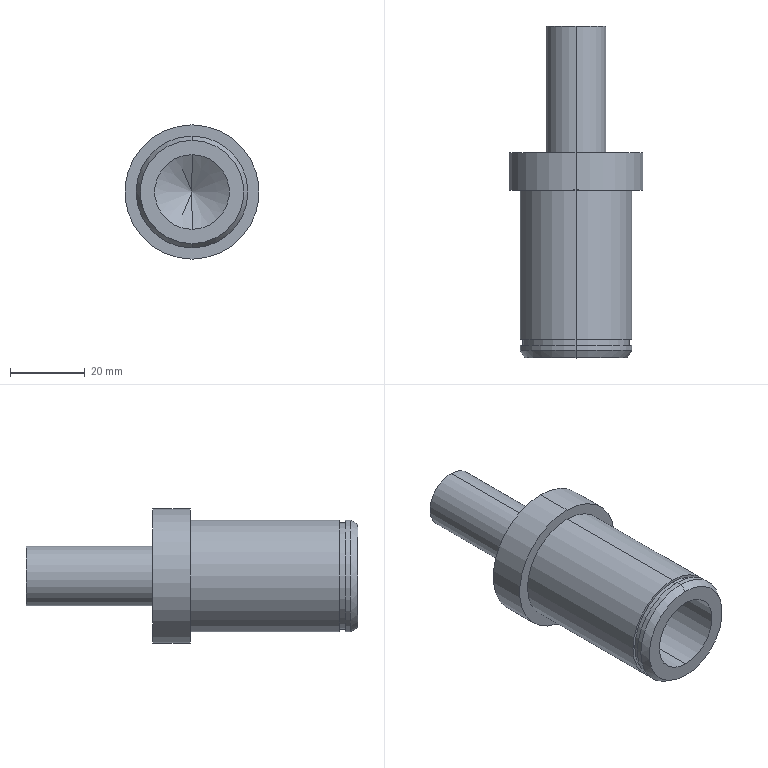Part | STEP file | 0229_221_Pin | 1 solid | 22 faces | box 36 x 89 x 36 mm | volume 38557 mm3 | cylinder 12 | plane 6 | cone 4 | commonest cylinder face diameters 30 x4 16 x2 20 x2 28.6 x2 36 x2
STEP:
#1=CARTESIAN_POINT('',(0.,0.,0.));
#2=DIRECTION('',(0.,0.,1.));
#3=DIRECTION('',(1.,0.,0.));
#4=AXIS2_PLACEMENT_3D('',#1,#2,#3);
#5=CARTESIAN_POINT('',(0.,-55.,-13.845));
#6=VERTEX_POINT('',#5);
#7=CARTESIAN_POINT('',(0.,-55.,13.845));
#8=VERTEX_POINT('',#7);
#9=CARTESIAN_POINT('',(0.,-55.,0.));
#10=DIRECTION('',(0.,-1.,0.));
#11=DIRECTION('',(0.,0.,1.));
#12=AXIS2_PLACEMENT_3D('',#9,#10,#11);
#13=CIRCLE('',#12,13.845);
#14=CARTESIAN_POINT('',(0.,-55.,0.));
#15=DIRECTION('',(0.,1.,0.));
#16=DIRECTION('',(0.,0.,1.));
#17=AXIS2_PLACEMENT_3D('',#14,#15,#16);
#18=CONICAL_SURFACE('',#17,13.845,0.5236);
#19=CARTESIAN_POINT('',(6.283,0.));
#20=DIRECTION('',(-1.,0.));
#21=VECTOR('',#20,1.);
#22=LINE('',#19,#21);
#23=(GEOMETRIC_REPRESENTATION_CONTEXT(2)PARAMETRIC_REPRESENTATION_CONTEXT()REPRESENTATION_CONTEXT('',''));
#24=DEFINITIONAL_REPRESENTATION('',(#22),#23);
#25=PCURVE('',#18,#24);
#26=CARTESIAN_POINT('',(-15.,-55.,0.));
#27=DIRECTION('',(0.,1.,0.));
#28=DIRECTION('',(0.,0.,1.));
#29=AXIS2_PLACEMENT_3D('',#26,#27,#28);
#30=PLANE('',#29);
#31=CARTESIAN_POINT('',(13.845,15.));
#32=CARTESIAN_POINT('',(13.845,-8.981));
#33=CARTESIAN_POINT('',(-6.923,3.01));
#34=CARTESIAN_POINT('',(-27.691,15.));
#35=CARTESIAN_POINT('',(-6.923,26.99));
#36=CARTESIAN_POINT('',(13.845,38.981));
#37=CARTESIAN_POINT('',(13.845,15.));
#38=(BOUNDED_CURVE()B_SPLINE_CURVE(2,(#31,#32,#33,#34,#35,#36,#37),.UNSPECIFIED.,.T.,.F.)B_SPLINE_CURVE_WITH_KNOTS((1,2,2,2,2,1),(-2.094,0.,2.094,4.189,6.283,8.378),.UNSPECIFIED.)CURVE()GEOMETRIC_REPRESENTATION_ITEM()RATIONAL_B_SPLINE_CURVE((1.,0.5,1.,0.5,1.,0.5,1.))REPRESENTATION_ITEM(''));
#39=(GEOMETRIC_REPRESENTATION_CONTEXT(2)PARAMETRIC_REPRESENTATION_CONTEXT()REPRESENTATION_CONTEXT('',''));
#40=DEFINITIONAL_REPRESENTATION('',(#38),#39);
#41=PCURVE('',#30,#40);
#42=SURFACE_CURVE('',#13,(#25,#41),.PCURVE_S1.);
#43=EDGE_CURVE('',#6,#8,#42,.T.);
#44=ORIENTED_EDGE('',*,*,#43,.F.);
#45=CARTESIAN_POINT('',(0.,-53.,-15.));
#46=VERTEX_POINT('',#45);
#47=CARTESIAN_POINT('',(0.,-55.,-13.845));
#48=DIRECTION('',(0.,0.866,-0.5));
#49=VECTOR('',#48,1.);
#50=LINE('',#47,#49);
#51=CARTESIAN_POINT('',(3.142,0.));
#52=DIRECTION('',(0.,1.));
#53=VECTOR('',#52,1.);
#54=LINE('',#51,#53);
#55=(GEOMETRIC_REPRESENTATION_CONTEXT(2)PARAMETRIC_REPRESENTATION_CONTEXT()REPRESENTATION_CONTEXT('',''));
#56=DEFINITIONAL_REPRESENTATION('',(#54),#55);
#57=PCURVE('',#18,#56);
#58=CARTESIAN_POINT('',(0.,-55.,0.));
#59=DIRECTION('',(0.,1.,0.));
#60=DIRECTION('',(0.,0.,1.));
#61=AXIS2_PLACEMENT_3D('',#58,#59,#60);
#62=CONICAL_SURFACE('',#61,13.845,0.5236);
#63=CARTESIAN_POINT('',(3.142,0.));
#64=DIRECTION('',(0.,1.));
#65=VECTOR('',#64,1.);
#66=LINE('',#63,#65);
#67=(GEOMETRIC_REPRESENTATION_CONTEXT(2)PARAMETRIC_REPRESENTATION_CONTEXT()REPRESENTATION_CONTEXT('',''));
#68=DEFINITIONAL_REPRESENTATION('',(#66),#67);
#69=PCURVE('',#62,#68);
#70=SURFACE_CURVE('',#50,(#57,#69),.PCURVE_S1.);
#71=EDGE_CURVE('',#6,#46,#70,.T.);
#72=ORIENTED_EDGE('',*,*,#71,.T.);
#73=CARTESIAN_POINT('',(0.,-53.,15.));
#74=VERTEX_POINT('',#73);
#75=CARTESIAN_POINT('',(0.,-53.,0.));
#76=DIRECTION('',(0.,1.,0.));
#77=DIRECTION('',(0.,0.,1.));
#78=AXIS2_PLACEMENT_3D('',#75,#76,#77);
#79=CIRCLE('',#78,15.);
#80=CARTESIAN_POINT('',(0.,2.));
#81=DIRECTION('',(1.,0.));
#82=VECTOR('',#81,1.);
#83=LINE('',#80,#82);
#84=(GEOMETRIC_REPRESENTATION_CONTEXT(2)PARAMETRIC_REPRESENTATION_CONTEXT()REPRESENTATION_CONTEXT('',''));
#85=DEFINITIONAL_REPRESENTATION('',(#83),#84);
#86=PCURVE('',#18,#85);
#87=CARTESIAN_POINT('',(0.,-62.558,0.));
#88=DIRECTION('',(0.,-1.,0.));
#89=DIRECTION('',(0.,0.,-1.));
#90=AXIS2_PLACEMENT_3D('',#87,#88,#89);
#91=CYLINDRICAL_SURFACE('',#90,15.);
#92=CARTESIAN_POINT('',(3.142,-9.558));
#93=DIRECTION('',(-1.,0.));
#94=VECTOR('',#93,1.);
#95=LINE('',#92,#94);
#96=(GEOMETRIC_REPRESENTATION_CONTEXT(2)PARAMETRIC_REPRESENTATION_CONTEXT()REPRESENTATION_CONTEXT('',''));
#97=DEFINITIONAL_REPRESENTATION('',(#95),#96);
#98=PCURVE('',#91,#97);
#99=SURFACE_CURVE('',#79,(#86,#98),.PCURVE_S1.);
#100=EDGE_CURVE('',#74,#46,#99,.T.);
#101=ORIENTED_EDGE('',*,*,#100,.F.);
#102=CARTESIAN_POINT('',(0.,-55.,13.845));
#103=DIRECTION('',(0.,0.866,0.5));
#104=VECTOR('',#103,1.);
#105=LINE('',#102,#104);
#106=CARTESIAN_POINT('',(0.,0.));
#107=DIRECTION('',(0.,1.));
#108=VECTOR('',#107,1.);
#109=LINE('',#106,#108);
#110=(GEOMETRIC_REPRESENTATION_CONTEXT(2)PARAMETRIC_REPRESENTATION_CONTEXT()REPRESENTATION_CONTEXT('',''));
#111=DEFINITIONAL_REPRESENTATION('',(#109),#110);
#112=PCURVE('',#18,#111);
#113=CARTESIAN_POINT('',(6.283,0.));
#114=DIRECTION('',(0.,1.));
#115=VECTOR('',#114,1.);
#116=LINE('',#113,#115);
#117=(GEOMETRIC_REPRESENTATION_CONTEXT(2)PARAMETRIC_REPRESENTATION_CONTEXT()REPRESENTATION_CONTEXT('',''));
#118=DEFINITIONAL_REPRESENTATION('',(#116),#117);
#119=PCURVE('',#62,#118);
#120=SURFACE_CURVE('',#105,(#112,#119),.PCURVE_S1.);
#121=EDGE_CURVE('',#8,#74,#120,.T.);
#122=ORIENTED_EDGE('',*,*,#121,.F.);
#123=EDGE_LOOP('',(#44,#72,#101,#122));
#124=FACE_BOUND('',#123,.T.);
#125=ADVANCED_FACE('',(#124),#18,.T.);
#126=CARTESIAN_POINT('',(0.,-25.,-10.));
#127=VERTEX_POINT('',#126);
#128=CARTESIAN_POINT('',(0.,-55.,-10.));
#129=VERTEX_POINT('',#128);
#130=CARTESIAN_POINT('',(0.,-55.,-10.));
#131=DIRECTION('',(0.,-1.,0.));
#132=VECTOR('',#131,1.);
#133=LINE('',#130,#132);
#134=CARTESIAN_POINT('',(0.,-55.,0.));
#135=DIRECTION('',(0.,-1.,0.));
#136=DIRECTION('',(0.,0.,-1.));
#137=AXIS2_PLACEMENT_3D('',#134,#135,#136);
#138=CYLINDRICAL_SURFACE('',#137,10.);
#139=CARTESIAN_POINT('',(6.283,0.));
#140=DIRECTION('',(0.,1.));
#141=VECTOR('',#140,1.);
#142=LINE('',#139,#141);
#143=(GEOMETRIC_REPRESENTATION_CONTEXT(2)PARAMETRIC_REPRESENTATION_CONTEXT()REPRESENTATION_CONTEXT('',''));
#144=DEFINITIONAL_REPRESENTATION('',(#142),#143);
#145=PCURVE('',#138,#144);
#146=CARTESIAN_POINT('',(0.,-55.,0.));
#147=DIRECTION('',(0.,-1.,0.));
#148=DIRECTION('',(0.,0.,-1.));
#149=AXIS2_PLACEMENT_3D('',#146,#147,#148);
#150=CYLINDRICAL_SURFACE('',#149,10.);
#151=CARTESIAN_POINT('',(0.,0.));
#152=DIRECTION('',(0.,1.));
#153=VECTOR('',#152,1.);
#154=LINE('',#151,#153);
#155=(GEOMETRIC_REPRESENTATION_CONTEXT(2)PARAMETRIC_REPRESENTATION_CONTEXT()REPRESENTATION_CONTEXT('',''));
#156=DEFINITIONAL_REPRESENTATION('',(#154),#155);
#157=PCURVE('',#150,#156);
#158=SURFACE_CURVE('',#133,(#145,#157),.PCURVE_S1.);
#159=EDGE_CURVE('',#127,#129,#158,.T.);
#160=ORIENTED_EDGE('',*,*,#159,.T.);
#161=CARTESIAN_POINT('',(0.,-55.,10.));
#162=VERTEX_POINT('',#161);
#163=CARTESIAN_POINT('',(0.,-55.,0.));
#164=DIRECTION('',(0.,-1.,0.));
#165=DIRECTION('',(0.,0.,-1.));
#166=AXIS2_PLACEMENT_3D('',#163,#164,#165);
#167=CIRCLE('',#166,10.);
#168=CARTESIAN_POINT('',(0.,0.));
#169=DIRECTION('',(1.,0.));
#170=VECTOR('',#169,1.);
#171=LINE('',#168,#170);
#172=(GEOMETRIC_REPRESENTATION_CONTEXT(2)PARAMETRIC_REPRESENTATION_CONTEXT()REPRESENTATION_CONTEXT('',''));
#173=DEFINITIONAL_REPRESENTATION('',(#171),#172);
#174=PCURVE('',#138,#173);
#175=CARTESIAN_POINT('',(-10.,15.));
#176=CARTESIAN_POINT('',(-10.,32.321));
#177=CARTESIAN_POINT('',(5.,23.66));
#178=CARTESIAN_POINT('',(20.,15.));
#179=CARTESIAN_POINT('',(5.,6.34));
#180=CARTESIAN_POINT('',(-10.,-2.321));
#181=CARTESIAN_POINT('',(-10.,15.));
#182=(BOUNDED_CURVE()B_SPLINE_CURVE(2,(#175,#176,#177,#178,#179,#180,#181),.UNSPECIFIED.,.T.,.F.)B_SPLINE_CURVE_WITH_KNOTS((1,2,2,2,2,1),(-2.094,0.,2.094,4.189,6.283,8.378),.UNSPECIFIED.)CURVE()GEOMETRIC_REPRESENTATION_ITEM()RATIONAL_B_SPLINE_CURVE((1.,0.5,1.,0.5,1.,0.5,1.))REPRESENTATION_ITEM(''));
#183=(GEOMETRIC_REPRESENTATION_CONTEXT(2)PARAMETRIC_REPRESENTATION_CONTEXT()REPRESENTATION_CONTEXT('',''));
#184=DEFINITIONAL_REPRESENTATION('',(#182),#183);
#185=PCURVE('',#30,#184);
#186=SURFACE_CURVE('',#167,(#174,#185),.PCURVE_S1.);
#187=EDGE_CURVE('',#162,#129,#186,.T.);
#188=ORIENTED_EDGE('',*,*,#187,.F.);
#189=CARTESIAN_POINT('',(0.,-25.,10.));
#190=VERTEX_POINT('',#189);
#191=CARTESIAN_POINT('',(0.,-55.,10.));
#192=DIRECTION('',(0.,-1.,0.));
#193=VECTOR('',#192,1.);
#194=LINE('',#191,#193);
#195=CARTESIAN_POINT('',(3.142,0.));
#196=DIRECTION('',(0.,1.));
#197=VECTOR('',#196,1.);
#198=LINE('',#195,#197);
#199=(GEOMETRIC_REPRESENTATION_CONTEXT(2)PARAMETRIC_REPRESENTATION_CONTEXT()REPRESENTATION_CONTEXT('',''));
#200=DEFINITIONAL_REPRESENTATION('',(#198),#199);
#201=PCURVE('',#138,#200);
#202=CARTESIAN_POINT('',(3.142,0.));
#203=DIRECTION('',(0.,1.));
#204=VECTOR('',#203,1.);
#205=LINE('',#202,#204);
#206=(GEOMETRIC_REPRESENTATION_CONTEXT(2)PARAMETRIC_REPRESENTATION_CONTEXT()REPRESENTATION_CONTEXT('',''));
#207=DEFINITIONAL_REPRESENTATION('',(#205),#206);
#208=PCURVE('',#150,#207);
#209=SURFACE_CURVE('',#194,(#201,#208),.PCURVE_S1.);
#210=EDGE_CURVE('',#190,#162,#209,.T.);
#211=ORIENTED_EDGE('',*,*,#210,.F.);
#212=CARTESIAN_POINT('',(0.,-25.,0.));
#213=DIRECTION('',(0.,-1.,0.));
#214=DIRECTION('',(0.,0.,-1.));
#215=AXIS2_PLACEMENT_3D('',#212,#213,#214);
#216=CIRCLE('',#215,10.);
#217=CARTESIAN_POINT('',(0.,-30.));
#218=DIRECTION('',(1.,0.));
#219=VECTOR('',#218,1.);
#220=LINE('',#217,#219);
#221=(GEOMETRIC_REPRESENTATION_CONTEXT(2)PARAMETRIC_REPRESENTATION_CONTEXT()REPRESENTATION_CONTEXT('',''));
#222=DEFINITIONAL_REPRESENTATION('',(#220),#221);
#223=PCURVE('',#138,#222);
#224=CARTESIAN_POINT('',(0.,-25.,0.));
#225=DIRECTION('',(0.,-1.,0.));
#226=DIRECTION('',(0.,0.,-1.));
#227=AXIS2_PLACEMENT_3D('',#224,#225,#226);
#228=CONICAL_SURFACE('',#227,10.,1.03);
#229=CARTESIAN_POINT('',(0.,0.));
#230=DIRECTION('',(1.,0.));
#231=VECTOR('',#230,1.);
#232=LINE('',#229,#231);
#233=(GEOMETRIC_REPRESENTATION_CONTEXT(2)PARAMETRIC_REPRESENTATION_CONTEXT()REPRESENTATION_CONTEXT('',''));
#234=DEFINITIONAL_REPRESENTATION('',(#232),#233);
#235=PCURVE('',#228,#234);
#236=SURFACE_CURVE('',#216,(#223,#235),.PCURVE_S1.);
#237=EDGE_CURVE('',#190,#127,#236,.T.);
#238=ORIENTED_EDGE('',*,*,#237,.T.);
#239=EDGE_LOOP('',(#160,#188,#211,#238));
#240=FACE_BOUND('',#239,.F.);
#241=ADVANCED_FACE('',(#240),#138,.F.);
#242=ORIENTED_EDGE('',*,*,#237,.F.);
#243=CARTESIAN_POINT('',(0.,-18.991,0.));
#244=VERTEX_POINT('',#243);
#245=CARTESIAN_POINT('',(0.,-25.,10.));
#246=DIRECTION('',(0.,-0.515,0.8572));
#247=VECTOR('',#246,1.);
#248=LINE('',#245,#247);
#249=CARTESIAN_POINT('',(3.142,0.));
#250=DIRECTION('',(0.,1.));
#251=VECTOR('',#250,1.);
#252=LINE('',#249,#251);
#253=(GEOMETRIC_REPRESENTATION_CONTEXT(2)PARAMETRIC_REPRESENTATION_CONTEXT()REPRESENTATION_CONTEXT('',''));
#254=DEFINITIONAL_REPRESENTATION('',(#252),#253);
#255=PCURVE('',#228,#254);
#256=CARTESIAN_POINT('',(0.,-25.,0.));
#257=DIRECTION('',(0.,-1.,0.));
#258=DIRECTION('',(0.,0.,-1.));
#259=AXIS2_PLACEMENT_3D('',#256,#257,#258);
#260=CONICAL_SURFACE('',#259,10.,1.03);
#261=CARTESIAN_POINT('',(3.142,0.));
#262=DIRECTION('',(0.,1.));
#263=VECTOR('',#262,1.);
#264=LINE('',#261,#263);
#265=(GEOMETRIC_REPRESENTATION_CONTEXT(2)PARAMETRIC_REPRESENTATION_CONTEXT()REPRESENTATION_CONTEXT('',''));
#266=DEFINITIONAL_REPRESENTATION('',(#264),#265);
#267=PCURVE('',#260,#266);
#268=SURFACE_CURVE('',#248,(#255,#267),.PCURVE_S1.);
#269=EDGE_CURVE('',#244,#190,#268,.T.);
#270=ORIENTED_EDGE('',*,*,#269,.F.);
#271=CARTESIAN_POINT('',(0.,-25.,-10.));
#272=DIRECTION('',(0.,-0.515,-0.8572));
#273=VECTOR('',#272,1.);
#274=LINE('',#271,#273);
#275=CARTESIAN_POINT('',(6.283,0.));
#276=DIRECTION('',(0.,1.));
#277=VECTOR('',#276,1.);
#278=LINE('',#275,#277);
#279=(GEOMETRIC_REPRESENTATION_CONTEXT(2)PARAMETRIC_REPRESENTATION_CONTEXT()REPRESENTATION_CONTEXT('',''));
#280=DEFINITIONAL_REPRESENTATION('',(#278),#279);
#281=PCURVE('',#228,#280);
#282=CARTESIAN_POINT('',(0.,0.));
#283=DIRECTION('',(0.,1.));
#284=VECTOR('',#283,1.);
#285=LINE('',#282,#284);
#286=(GEOMETRIC_REPRESENTATION_CONTEXT(2)PARAMETRIC_REPRESENTATION_CONTEXT()REPRESENTATION_CONTEXT('',''));
#287=DEFINITIONAL_REPRESENTATION('',(#285),#286);
#288=PCURVE('',#260,#287);
#289=SURFACE_CURVE('',#274,(#281,#288),.PCURVE_S1.);
#290=EDGE_CURVE('',#244,#127,#289,.T.);
#291=ORIENTED_EDGE('',*,*,#290,.T.);
#292=EDGE_LOOP('',(#242,#270,#291));
#293=FACE_BOUND('',#292,.F.);
#294=ADVANCED_FACE('',(#293),#228,.F.);
#295=CARTESIAN_POINT('',(0.,-10.,-15.));
#296=VERTEX_POINT('',#295);
#297=CARTESIAN_POINT('',(0.,-10.,15.));
#298=VERTEX_POINT('',#297);
#299=CARTESIAN_POINT('',(0.,-10.,0.));
#300=DIRECTION('',(0.,-1.,0.));
#301=DIRECTION('',(0.,0.,-1.));
#302=AXIS2_PLACEMENT_3D('',#299,#300,#301);
#303=CIRCLE('',#302,15.);
#304=CARTESIAN_POINT('',(0.,-62.558,0.));
#305=DIRECTION('',(0.,-1.,0.));
#306=DIRECTION('',(0.,0.,-1.));
#307=AXIS2_PLACEMENT_3D('',#304,#305,#306);
#308=CYLINDRICAL_SURFACE('',#307,15.);
#309=CARTESIAN_POINT('',(0.,-52.558));
#310=DIRECTION('',(1.,0.));
#311=VECTOR('',#310,1.);
#312=LINE('',#309,#311);
#313=(GEOMETRIC_REPRESENTATION_CONTEXT(2)PARAMETRIC_REPRESENTATION_CONTEXT()REPRESENTATION_CONTEXT('',''));
#314=DEFINITIONAL_REPRESENTATION('',(#312),#313);
#315=PCURVE('',#308,#314);
#316=CARTESIAN_POINT('',(-15.,-10.,0.));
#317=DIRECTION('',(0.,1.,0.));
#318=DIRECTION('',(0.,0.,1.));
#319=AXIS2_PLACEMENT_3D('',#316,#317,#318);
#320=PLANE('',#319);
#321=CARTESIAN_POINT('',(-15.,15.));
#322=CARTESIAN_POINT('',(-15.,40.981));
#323=CARTESIAN_POINT('',(7.5,27.99));
#324=CARTESIAN_POINT('',(30.,15.));
#325=CARTESIAN_POINT('',(7.5,2.01));
#326=CARTESIAN_POINT('',(-15.,-10.981));
#327=CARTESIAN_POINT('',(-15.,15.));
#328=(BOUNDED_CURVE()B_SPLINE_CURVE(2,(#321,#322,#323,#324,#325,#326,#327),.UNSPECIFIED.,.T.,.F.)B_SPLINE_CURVE_WITH_KNOTS((1,2,2,2,2,1),(-2.094,0.,2.094,4.189,6.283,8.378),.UNSPECIFIED.)CURVE()GEOMETRIC_REPRESENTATION_ITEM()RATIONAL_B_SPLINE_CURVE((1.,0.5,1.,0.5,1.,0.5,1.))REPRESENTATION_ITEM(''));
#329=(GEOMETRIC_REPRESENTATION_CONTEXT(2)PARAMETRIC_REPRESENTATION_CONTEXT()REPRESENTATION_CONTEXT('',''));
#330=DEFINITIONAL_REPRESENTATION('',(#328),#329);
#331=PCURVE('',#320,#330);
#332=SURFACE_CURVE('',#303,(#315,#331),.PCURVE_S1.);
#333=EDGE_CURVE('',#296,#298,#332,.T.);
#334=ORIENTED_EDGE('',*,*,#333,.T.);
#335=CARTESIAN_POINT('',(0.,-50.,15.));
#336=VERTEX_POINT('',#335);
#337=CARTESIAN_POINT('',(0.,-62.558,15.));
#338=DIRECTION('',(0.,-1.,0.));
#339=VECTOR('',#338,1.);
#340=LINE('',#337,#339);
#341=CARTESIAN_POINT('',(3.142,0.));
#342=DIRECTION('',(0.,1.));
#343=VECTOR('',#342,1.);
#344=LINE('',#341,#343);
#345=(GEOMETRIC_REPRESENTATION_CONTEXT(2)PARAMETRIC_REPRESENTATION_CONTEXT()REPRESENTATION_CONTEXT('',''));
#346=DEFINITIONAL_REPRESENTATION('',(#344),#345);
#347=PCURVE('',#308,#346);
#348=CARTESIAN_POINT('',(0.,-62.558,0.));
#349=DIRECTION('',(0.,-1.,0.));
#350=DIRECTION('',(0.,0.,-1.));
#351=AXIS2_PLACEMENT_3D('',#348,#349,#350);
#352=CYLINDRICAL_SURFACE('',#351,15.);
#353=CARTESIAN_POINT('',(3.142,0.));
#354=DIRECTION('',(0.,1.));
#355=VECTOR('',#354,1.);
#356=LINE('',#353,#355);
#357=(GEOMETRIC_REPRESENTATION_CONTEXT(2)PARAMETRIC_REPRESENTATION_CONTEXT()REPRESENTATION_CONTEXT('',''));
#358=DEFINITIONAL_REPRESENTATION('',(#356),#357);
#359=PCURVE('',#352,#358);
#360=SURFACE_CURVE('',#340,(#347,#359),.PCURVE_S1.);
#361=EDGE_CURVE('',#298,#336,#360,.T.);
#362=ORIENTED_EDGE('',*,*,#361,.T.);
#363=CARTESIAN_POINT('',(0.,-50.,-15.));
#364=VERTEX_POINT('',#363);
#365=CARTESIAN_POINT('',(0.,-50.,0.));
#366=DIRECTION('',(0.,-1.,0.));
#367=DIRECTION('',(0.,0.,-1.));
#368=AXIS2_PLACEMENT_3D('',#365,#366,#367);
#369=CIRCLE('',#368,15.);
#370=CARTESIAN_POINT('',(0.,-12.558));
#371=DIRECTION('',(1.,0.));
#372=VECTOR('',#371,1.);
#373=LINE('',#370,#372);
#374=(GEOMETRIC_REPRESENTATION_CONTEXT(2)PARAMETRIC_REPRESENTATION_CONTEXT()REPRESENTATION_CONTEXT('',''));
#375=DEFINITIONAL_REPRESENTATION('',(#373),#374);
#376=PCURVE('',#308,#375);
#377=CARTESIAN_POINT('',(-15.,-50.,0.));
#378=DIRECTION('',(0.,1.,0.));
#379=DIRECTION('',(0.,0.,1.));
#380=AXIS2_PLACEMENT_3D('',#377,#378,#379);
#381=PLANE('',#380);
#382=CARTESIAN_POINT('',(-15.,15.));
#383=CARTESIAN_POINT('',(-15.,40.981));
#384=CARTESIAN_POINT('',(7.5,27.99));
#385=CARTESIAN_POINT('',(30.,15.));
#386=CARTESIAN_POINT('',(7.5,2.01));
#387=CARTESIAN_POINT('',(-15.,-10.981));
#388=CARTESIAN_POINT('',(-15.,15.));
#389=(BOUNDED_CURVE()B_SPLINE_CURVE(2,(#382,#383,#384,#385,#386,#387,#388),.UNSPECIFIED.,.T.,.F.)B_SPLINE_CURVE_WITH_KNOTS((1,2,2,2,2,1),(-2.094,0.,2.094,4.189,6.283,8.378),.UNSPECIFIED.)CURVE()GEOMETRIC_REPRESENTATION_ITEM()RATIONAL_B_SPLINE_CURVE((1.,0.5,1.,0.5,1.,0.5,1.))REPRESENTATION_ITEM(''));
#390=(GEOMETRIC_REPRESENTATION_CONTEXT(2)PARAMETRIC_REPRESENTATION_CONTEXT()REPRESENTATION_CONTEXT('',''));
#391=DEFINITIONAL_REPRESENTATION('',(#389),#390);
#392=PCURVE('',#381,#391);
#393=SURFACE_CURVE('',#369,(#376,#392),.PCURVE_S1.);
#394=EDGE_CURVE('',#364,#336,#393,.T.);
#395=ORIENTED_EDGE('',*,*,#394,.F.);
#396=CARTESIAN_POINT('',(0.,-62.558,-15.));
#397=DIRECTION('',(0.,-1.,0.));
#398=VECTOR('',#397,1.);
#399=LINE('',#396,#398);
#400=CARTESIAN_POINT('',(0.,0.));
#401=DIRECTION('',(0.,1.));
#402=VECTOR('',#401,1.);
#403=LINE('',#400,#402);
#404=(GEOMETRIC_REPRESENTATION_CONTEXT(2)PARAMETRIC_REPRESENTATION_CONTEXT()REPRESENTATION_CONTEXT('',''));
#405=DEFINITIONAL_REPRESENTATION('',(#403),#404);
#406=PCURVE('',#308,#405);
#407=CARTESIAN_POINT('',(6.283,0.));
#408=DIRECTION('',(0.,1.));
#409=VECTOR('',#408,1.);
#410=LINE('',#407,#409);
#411=(GEOMETRIC_REPRESENTATION_CONTEXT(2)PARAMETRIC_REPRESENTATION_CONTEXT()REPRESENTATION_CONTEXT('',''));
#412=DEFINITIONAL_REPRESENTATION('',(#410),#411);
#413=PCURVE('',#352,#412);
#414=SURFACE_CURVE('',#399,(#406,#413),.PCURVE_S1.);
#415=EDGE_CURVE('',#296,#364,#414,.T.);
#416=ORIENTED_EDGE('',*,*,#415,.F.);
#417=EDGE_LOOP('',(#334,#362,#395,#416));
#418=FACE_BOUND('',#417,.T.);
#419=ADVANCED_FACE('',(#418),#308,.T.);
#420=CARTESIAN_POINT('',(0.,-50.,-14.3));
#421=VERTEX_POINT('',#420);
#422=CARTESIAN_POINT('',(0.,-50.,14.3));
#423=VERTEX_POINT('',#422);
#424=CARTESIAN_POINT('',(0.,-50.,0.));
#425=DIRECTION('',(0.,-1.,0.));
#426=DIRECTION('',(0.,0.,-1.));
#427=AXIS2_PLACEMENT_3D('',#424,#425,#426);
#428=CIRCLE('',#427,14.3);
#429=CARTESIAN_POINT('',(0.,-62.558,0.));
#430=DIRECTION('',(0.,-1.,0.));
#431=DIRECTION('',(0.,0.,-1.));
#432=AXIS2_PLACEMENT_3D('',#429,#430,#431);
#433=CYLINDRICAL_SURFACE('',#432,14.3);
#434=CARTESIAN_POINT('',(0.,-12.558));
#435=DIRECTION('',(1.,0.));
#436=VECTOR('',#435,1.);
#437=LINE('',#434,#436);
#438=(GEOMETRIC_REPRESENTATION_CONTEXT(2)PARAMETRIC_REPRESENTATION_CONTEXT()REPRESENTATION_CONTEXT('',''));
#439=DEFINITIONAL_REPRESENTATION('',(#437),#438);
#440=PCURVE('',#433,#439);
#441=CARTESIAN_POINT('',(-14.3,15.));
#442=CARTESIAN_POINT('',(-14.3,39.768));
#443=CARTESIAN_POINT('',(7.15,27.384));
#444=CARTESIAN_POINT('',(28.6,15.));
#445=CARTESIAN_POINT('',(7.15,2.616));
#446=CARTESIAN_POINT('',(-14.3,-9.768));
#447=CARTESIAN_POINT('',(-14.3,15.));
#448=(BOUNDED_CURVE()B_SPLINE_CURVE(2,(#441,#442,#443,#444,#445,#446,#447),.UNSPECIFIED.,.T.,.F.)B_SPLINE_CURVE_WITH_KNOTS((1,2,2,2,2,1),(-2.094,0.,2.094,4.189,6.283,8.378),.UNSPECIFIED.)CURVE()GEOMETRIC_REPRESENTATION_ITEM()RATIONAL_B_SPLINE_CURVE((1.,0.5,1.,0.5,1.,0.5,1.))REPRESENTATION_ITEM(''));
#449=(GEOMETRIC_REPRESENTATION_CONTEXT(2)PARAMETRIC_REPRESENTATION_CONTEXT()REPRESENTATION_CONTEXT('',''));
#450=DEFINITIONAL_REPRESENTATION('',(#448),#449);
#451=PCURVE('',#381,#450);
#452=SURFACE_CURVE('',#428,(#440,#451),.PCURVE_S1.);
#453=EDGE_CURVE('',#421,#423,#452,.T.);
#454=ORIENTED_EDGE('',*,*,#453,.T.);
#455=CARTESIAN_POINT('',(0.,-51.65,14.3));
#456=VERTEX_POINT('',#455);
#457=CARTESIAN_POINT('',(0.,-62.558,14.3));
#458=DIRECTION('',(0.,-1.,0.));
#459=VECTOR('',#458,1.);
#460=LINE('',#457,#459);
#461=CARTESIAN_POINT('',(3.142,0.));
#462=DIRECTION('',(0.,1.));
#463=VECTOR('',#462,1.);
#464=LINE('',#461,#463);
#465=(GEOMETRIC_REPRESENTATION_CONTEXT(2)PARAMETRIC_REPRESENTATION_CONTEXT()REPRESENTATION_CONTEXT('',''));
#466=DEFINITIONAL_REPRESENTATION('',(#464),#465);
#467=PCURVE('',#433,#466);
#468=CARTESIAN_POINT('',(0.,-62.558,0.));
#469=DIRECTION('',(0.,-1.,0.));
#470=DIRECTION('',(0.,0.,-1.));
#471=AXIS2_PLACEMENT_3D('',#468,#469,#470);
#472=CYLINDRICAL_SURFACE('',#471,14.3);
#473=CARTESIAN_POINT('',(3.142,0.));
#474=DIRECTION('',(0.,1.));
#475=VECTOR('',#474,1.);
#476=LINE('',#473,#475);
#477=(GEOMETRIC_REPRESENTATION_CONTEXT(2)PARAMETRIC_REPRESENTATION_CONTEXT()REPRESENTATION_CONTEXT('',''));
#478=DEFINITIONAL_REPRESENTATION('',(#476),#477);
#479=PCURVE('',#472,#478);
#480=SURFACE_CURVE('',#460,(#467,#479),.PCURVE_S1.);
#481=EDGE_CURVE('',#423,#456,#480,.T.);
#482=ORIENTED_EDGE('',*,*,#481,.T.);
#483=CARTESIAN_POINT('',(0.,-51.65,-14.3));
#484=VERTEX_POINT('',#483);
#485=CARTESIAN_POINT('',(0.,-51.65,0.));
#486=DIRECTION('',(0.,-1.,0.));
#487=DIRECTION('',(0.,0.,-1.));
#488=AXIS2_PLACEMENT_3D('',#485,#486,#487);
#489=CIRCLE('',#488,14.3);
#490=CARTESIAN_POINT('',(0.,-10.908));
#491=DIRECTION('',(1.,0.));
#492=VECTOR('',#491,1.);
#493=LINE('',#490,#492);
#494=(GEOMETRIC_REPRESENTATION_CONTEXT(2)PARAMETRIC_REPRESENTATION_CONTEXT()REPRESENTATION_CONTEXT('',''));
#495=DEFINITIONAL_REPRESENTATION('',(#493),#494);
#496=PCURVE('',#433,#495);
#497=CARTESIAN_POINT('',(-15.,-51.65,0.));
#498=DIRECTION('',(0.,-1.,0.));
#499=DIRECTION('',(0.,0.,-1.));
#500=AXIS2_PLACEMENT_3D('',#497,#498,#499);
#501=PLANE('',#500);
#502=CARTESIAN_POINT('',(0.,15.));
#503=DIRECTION('',(1.,0.));
#504=AXIS2_PLACEMENT_2D('',#502,#503);
#505=CIRCLE('',#504,14.3);
#506=(GEOMETRIC_REPRESENTATION_CONTEXT(2)PARAMETRIC_REPRESENTATION_CONTEXT()REPRESENTATION_CONTEXT('',''));
#507=DEFINITIONAL_REPRESENTATION('',(#505),#506);
#508=PCURVE('',#501,#507);
#509=SURFACE_CURVE('',#489,(#496,#508),.PCURVE_S1.);
#510=EDGE_CURVE('',#484,#456,#509,.T.);
#511=ORIENTED_EDGE('',*,*,#510,.F.);
#512=CARTESIAN_POINT('',(0.,-62.558,-14.3));
#513=DIRECTION('',(0.,-1.,0.));
#514=VECTOR('',#513,1.);
#515=LINE('',#512,#514);
#516=CARTESIAN_POINT('',(0.,0.));
#517=DIRECTION('',(0.,1.));
#518=VECTOR('',#517,1.);
#519=LINE('',#516,#518);
#520=(GEOMETRIC_REPRESENTATION_CONTEXT(2)PARAMETRIC_REPRESENTATION_CONTEXT()REPRESENTATION_CONTEXT('',''));
#521=DEFINITIONAL_REPRESENTATION('',(#519),#520);
#522=PCURVE('',#433,#521);
#523=CARTESIAN_POINT('',(6.283,0.));
#524=DIRECTION('',(0.,1.));
#525=VECTOR('',#524,1.);
#526=LINE('',#523,#525);
#527=(GEOMETRIC_REPRESENTATION_CONTEXT(2)PARAMETRIC_REPRESENTATION_CONTEXT()REPRESENTATION_CONTEXT('',''));
#528=DEFINITIONAL_REPRESENTATION('',(#526),#527);
#529=PCURVE('',#472,#528);
#530=SURFACE_CURVE('',#515,(#522,#529),.PCURVE_S1.);
#531=EDGE_CURVE('',#421,#484,#530,.T.);
#532=ORIENTED_EDGE('',*,*,#531,.F.);
#533=EDGE_LOOP('',(#454,#482,#511,#532));
#534=FACE_BOUND('',#533,.T.);
#535=ADVANCED_FACE('',(#534),#433,.T.);
#536=CARTESIAN_POINT('',(0.,-51.65,-15.));
#537=VERTEX_POINT('',#536);
#538=CARTESIAN_POINT('',(0.,-51.65,15.));
#539=VERTEX_POINT('',#538);
#540=CARTESIAN_POINT('',(0.,-51.65,0.));
#541=DIRECTION('',(0.,-1.,0.));
#542=DIRECTION('',(0.,0.,-1.));
#543=AXIS2_PLACEMENT_3D('',#540,#541,#542);
#544=CIRCLE('',#543,15.);
#545=CARTESIAN_POINT('',(0.,-10.908));
#546=DIRECTION('',(1.,0.));
#547=VECTOR('',#546,1.);
#548=LINE('',#545,#547);
#549=(GEOMETRIC_REPRESENTATION_CONTEXT(2)PARAMETRIC_REPRESENTATION_CONTEXT()REPRESENTATION_CONTEXT('',''));
#550=DEFINITIONAL_REPRESENTATION('',(#548),#549);
#551=PCURVE('',#91,#550);
#552=CARTESIAN_POINT('',(0.,15.));
#553=DIRECTION('',(1.,0.));
#554=AXIS2_PLACEMENT_2D('',#552,#553);
#555=CIRCLE('',#554,15.);
#556=(GEOMETRIC_REPRESENTATION_CONTEXT(2)PARAMETRIC_REPRESENTATION_CONTEXT()REPRESENTATION_CONTEXT('',''));
#557=DEFINITIONAL_REPRESENTATION('',(#555),#556);
#558=PCURVE('',#501,#557);
#559=SURFACE_CURVE('',#544,(#551,#558),.PCURVE_S1.);
#560=EDGE_CURVE('',#537,#539,#559,.T.);
#561=ORIENTED_EDGE('',*,*,#560,.T.);
#562=CARTESIAN_POINT('',(0.,-62.558,15.));
#563=DIRECTION('',(0.,-1.,0.));
#564=VECTOR('',#563,1.);
#565=LINE('',#562,#564);
#566=CARTESIAN_POINT('',(3.142,0.));
#567=DIRECTION('',(0.,1.));
#568=VECTOR('',#567,1.);
#569=LINE('',#566,#568);
#570=(GEOMETRIC_REPRESENTATION_CONTEXT(2)PARAMETRIC_REPRESENTATION_CONTEXT()REPRESENTATION_CONTEXT('',''));
#571=DEFINITIONAL_REPRESENTATION('',(#569),#570);
#572=PCURVE('',#91,#571);
#573=CARTESIAN_POINT('',(0.,-62.558,0.));
#574=DIRECTION('',(0.,-1.,0.));
#575=DIRECTION('',(0.,0.,-1.));
#576=AXIS2_PLACEMENT_3D('',#573,#574,#575);
#577=CYLINDRICAL_SURFACE('',#576,15.);
#578=CARTESIAN_POINT('',(3.142,0.));
#579=DIRECTION('',(0.,1.));
#580=VECTOR('',#579,1.);
#581=LINE('',#578,#580);
#582=(GEOMETRIC_REPRESENTATION_CONTEXT(2)PARAMETRIC_REPRESENTATION_CONTEXT()REPRESENTATION_CONTEXT('',''));
#583=DEFINITIONAL_REPRESENTATION('',(#581),#582);
#584=PCURVE('',#577,#583);
#585=SURFACE_CURVE('',#565,(#572,#584),.PCURVE_S1.);
#586=EDGE_CURVE('',#539,#74,#585,.T.);
#587=ORIENTED_EDGE('',*,*,#586,.T.);
#588=ORIENTED_EDGE('',*,*,#100,.T.);
#589=CARTESIAN_POINT('',(0.,-62.558,-15.));
#590=DIRECTION('',(0.,-1.,0.));
#591=VECTOR('',#590,1.);
#592=LINE('',#589,#591);
#593=CARTESIAN_POINT('',(0.,0.));
#594=DIRECTION('',(0.,1.));
#595=VECTOR('',#594,1.);
#596=LINE('',#593,#595);
#597=(GEOMETRIC_REPRESENTATION_CONTEXT(2)PARAMETRIC_REPRESENTATION_CONTEXT()REPRESENTATION_CONTEXT('',''));
#598=DEFINITIONAL_REPRESENTATION('',(#596),#597);
#599=PCURVE('',#91,#598);
#600=CARTESIAN_POINT('',(6.283,0.));
#601=DIRECTION('',(0.,1.));
#602=VECTOR('',#601,1.);
#603=LINE('',#600,#602);
#604=(GEOMETRIC_REPRESENTATION_CONTEXT(2)PARAMETRIC_REPRESENTATION_CONTEXT()REPRESENTATION_CONTEXT('',''));
#605=DEFINITIONAL_REPRESENTATION('',(#603),#604);
#606=PCURVE('',#577,#605);
#607=SURFACE_CURVE('',#592,(#599,#606),.PCURVE_S1.);
#608=EDGE_CURVE('',#537,#46,#607,.T.);
#609=ORIENTED_EDGE('',*,*,#608,.F.);
#610=EDGE_LOOP('',(#561,#587,#588,#609));
#611=FACE_BOUND('',#610,.T.);
#612=ADVANCED_FACE('',(#611),#91,.T.);
#613=CARTESIAN_POINT('',(0.,34.,-8.));
#614=VERTEX_POINT('',#613);
#615=CARTESIAN_POINT('',(0.,34.,8.));
#616=VERTEX_POINT('',#615);
#617=CARTESIAN_POINT('',(0.,34.,0.));
#618=DIRECTION('',(0.,-1.,0.));
#619=DIRECTION('',(0.,0.,-1.));
#620=AXIS2_PLACEMENT_3D('',#617,#618,#619);
#621=CIRCLE('',#620,8.);
#622=CARTESIAN_POINT('',(0.,-62.558,0.));
#623=DIRECTION('',(0.,-1.,0.));
#624=DIRECTION('',(0.,0.,-1.));
#625=AXIS2_PLACEMENT_3D('',#622,#623,#624);
#626=CYLINDRICAL_SURFACE('',#625,8.);
#627=CARTESIAN_POINT('',(0.,-96.558));
#628=DIRECTION('',(1.,0.));
#629=VECTOR('',#628,1.);
#630=LINE('',#627,#629);
#631=(GEOMETRIC_REPRESENTATION_CONTEXT(2)PARAMETRIC_REPRESENTATION_CONTEXT()REPRESENTATION_CONTEXT('',''));
#632=DEFINITIONAL_REPRESENTATION('',(#630),#631);
#633=PCURVE('',#626,#632);
#634=CARTESIAN_POINT('',(0.,34.,0.));
#635=DIRECTION('',(0.,-1.,0.));
#636=DIRECTION('',(0.,0.,-1.));
#637=AXIS2_PLACEMENT_3D('',#634,#635,#636);
#638=PLANE('',#637);
#639=CARTESIAN_POINT('',(0.,0.));
#640=DIRECTION('',(1.,0.));
#641=AXIS2_PLACEMENT_2D('',#639,#640);
#642=CIRCLE('',#641,8.);
#643=(GEOMETRIC_REPRESENTATION_CONTEXT(2)PARAMETRIC_REPRESENTATION_CONTEXT()REPRESENTATION_CONTEXT('',''));
#644=DEFINITIONAL_REPRESENTATION('',(#642),#643);
#645=PCURVE('',#638,#644);
#646=SURFACE_CURVE('',#621,(#633,#645),.PCURVE_S1.);
#647=EDGE_CURVE('',#614,#616,#646,.T.);
#648=ORIENTED_EDGE('',*,*,#647,.T.);
#649=CARTESIAN_POINT('',(0.,0.,8.));
#650=VERTEX_POINT('',#649);
#651=CARTESIAN_POINT('',(0.,-62.558,8.));
#652=DIRECTION('',(0.,-1.,0.));
#653=VECTOR('',#652,1.);
#654=LINE('',#651,#653);
#655=CARTESIAN_POINT('',(3.142,0.));
#656=DIRECTION('',(0.,1.));
#657=VECTOR('',#656,1.);
#658=LINE('',#655,#657);
#659=(GEOMETRIC_REPRESENTATION_CONTEXT(2)PARAMETRIC_REPRESENTATION_CONTEXT()REPRESENTATION_CONTEXT('',''));
#660=DEFINITIONAL_REPRESENTATION('',(#658),#659);
#661=PCURVE('',#626,#660);
#662=CARTESIAN_POINT('',(0.,-62.558,0.));
#663=DIRECTION('',(0.,-1.,0.));
#664=DIRECTION('',(0.,0.,-1.));
#665=AXIS2_PLACEMENT_3D('',#662,#663,#664);
#666=CYLINDRICAL_SURFACE('',#665,8.);
#667=CARTESIAN_POINT('',(3.142,0.));
#668=DIRECTION('',(0.,1.));
#669=VECTOR('',#668,1.);
#670=LINE('',#667,#669);
#671=(GEOMETRIC_REPRESENTATION_CONTEXT(2)PARAMETRIC_REPRESENTATION_CONTEXT()REPRESENTATION_CONTEXT('',''));
#672=DEFINITIONAL_REPRESENTATION('',(#670),#671);
#673=PCURVE('',#666,#672);
#674=SURFACE_CURVE('',#654,(#661,#673),.PCURVE_S1.);
#675=EDGE_CURVE('',#616,#650,#674,.T.);
#676=ORIENTED_EDGE('',*,*,#675,.T.);
#677=CARTESIAN_POINT('',(0.,0.,-8.));
#678=VERTEX_POINT('',#677);
#679=CARTESIAN_POINT('',(0.,0.,0.));
#680=DIRECTION('',(0.,-1.,0.));
#681=DIRECTION('',(0.,0.,-1.));
#682=AXIS2_PLACEMENT_3D('',#679,#680,#681);
#683=CIRCLE('',#682,8.);
#684=CARTESIAN_POINT('',(0.,-62.558));
#685=DIRECTION('',(1.,0.));
#686=VECTOR('',#685,1.);
#687=LINE('',#684,#686);
#688=(GEOMETRIC_REPRESENTATION_CONTEXT(2)PARAMETRIC_REPRESENTATION_CONTEXT()REPRESENTATION_CONTEXT('',''));
#689=DEFINITIONAL_REPRESENTATION('',(#687),#688);
#690=PCURVE('',#626,#689);
#691=CARTESIAN_POINT('',(-8.,0.,0.));
#692=DIRECTION('',(0.,-1.,0.));
#693=DIRECTION('',(0.,0.,-1.));
#694=AXIS2_PLACEMENT_3D('',#691,#692,#693);
#695=PLANE('',#694);
#696=CARTESIAN_POINT('',(0.,8.));
#697=DIRECTION('',(1.,0.));
#698=AXIS2_PLACEMENT_2D('',#696,#697);
#699=CIRCLE('',#698,8.);
#700=(GEOMETRIC_REPRESENTATION_CONTEXT(2)PARAMETRIC_REPRESENTATION_CONTEXT()REPRESENTATION_CONTEXT('',''));
#701=DEFINITIONAL_REPRESENTATION('',(#699),#700);
#702=PCURVE('',#695,#701);
#703=SURFACE_CURVE('',#683,(#690,#702),.PCURVE_S1.);
#704=EDGE_CURVE('',#678,#650,#703,.T.);
#705=ORIENTED_EDGE('',*,*,#704,.F.);
#706=CARTESIAN_POINT('',(0.,-62.558,-8.));
#707=DIRECTION('',(0.,-1.,0.));
#708=VECTOR('',#707,1.);
#709=LINE('',#706,#708);
#710=CARTESIAN_POINT('',(0.,0.));
#711=DIRECTION('',(0.,1.));
#712=VECTOR('',#711,1.);
#713=LINE('',#710,#712);
#714=(GEOMETRIC_REPRESENTATION_CONTEXT(2)PARAMETRIC_REPRESENTATION_CONTEXT()REPRESENTATION_CONTEXT('',''));
#715=DEFINITIONAL_REPRESENTATION('',(#713),#714);
#716=PCURVE('',#626,#715);
#717=CARTESIAN_POINT('',(6.283,0.));
#718=DIRECTION('',(0.,1.));
#719=VECTOR('',#718,1.);
#720=LINE('',#717,#719);
#721=(GEOMETRIC_REPRESENTATION_CONTEXT(2)PARAMETRIC_REPRESENTATION_CONTEXT()REPRESENTATION_CONTEXT('',''));
#722=DEFINITIONAL_REPRESENTATION('',(#720),#721);
#723=PCURVE('',#666,#722);
#724=SURFACE_CURVE('',#709,(#716,#723),.PCURVE_S1.);
#725=EDGE_CURVE('',#614,#678,#724,.T.);
#726=ORIENTED_EDGE('',*,*,#725,.F.);
#727=EDGE_LOOP('',(#648,#676,#705,#726));
#728=FACE_BOUND('',#727,.T.);
#729=ADVANCED_FACE('',(#728),#626,.T.);
#730=CARTESIAN_POINT('',(0.,0.,-18.));
#731=VERTEX_POINT('',#730);
#732=CARTESIAN_POINT('',(0.,0.,18.));
#733=VERTEX_POINT('',#732);
#734=CARTESIAN_POINT('',(0.,0.,0.));
#735=DIRECTION('',(0.,-1.,0.));
#736=DIRECTION('',(0.,0.,-1.));
#737=AXIS2_PLACEMENT_3D('',#734,#735,#736);
#738=CIRCLE('',#737,18.);
#739=CARTESIAN_POINT('',(0.,-62.558,0.));
#740=DIRECTION('',(0.,-1.,0.));
#741=DIRECTION('',(0.,0.,-1.));
#742=AXIS2_PLACEMENT_3D('',#739,#740,#741);
#743=CYLINDRICAL_SURFACE('',#742,18.);
#744=CARTESIAN_POINT('',(0.,-62.558));
#745=DIRECTION('',(1.,0.));
#746=VECTOR('',#745,1.);
#747=LINE('',#744,#746);
#748=(GEOMETRIC_REPRESENTATION_CONTEXT(2)PARAMETRIC_REPRESENTATION_CONTEXT()REPRESENTATION_CONTEXT('',''));
#749=DEFINITIONAL_REPRESENTATION('',(#747),#748);
#750=PCURVE('',#743,#749);
#751=CARTESIAN_POINT('',(0.,8.));
#752=DIRECTION('',(1.,0.));
#753=AXIS2_PLACEMENT_2D('',#751,#752);
#754=CIRCLE('',#753,18.);
#755=(GEOMETRIC_REPRESENTATION_CONTEXT(2)PARAMETRIC_REPRESENTATION_CONTEXT()REPRESENTATION_CONTEXT('',''));
#756=DEFINITIONAL_REPRESENTATION('',(#754),#755);
#757=PCURVE('',#695,#756);
#758=SURFACE_CURVE('',#738,(#750,#757),.PCURVE_S1.);
#759=EDGE_CURVE('',#731,#733,#758,.T.);
#760=ORIENTED_EDGE('',*,*,#759,.T.);
#761=CARTESIAN_POINT('',(0.,-10.,18.));
#762=VERTEX_POINT('',#761);
#763=CARTESIAN_POINT('',(0.,-62.558,18.));
#764=DIRECTION('',(0.,-1.,0.));
#765=VECTOR('',#764,1.);
#766=LINE('',#763,#765);
#767=CARTESIAN_POINT('',(3.142,0.));
#768=DIRECTION('',(0.,1.));
#769=VECTOR('',#768,1.);
#770=LINE('',#767,#769);
#771=(GEOMETRIC_REPRESENTATION_CONTEXT(2)PARAMETRIC_REPRESENTATION_CONTEXT()REPRESENTATION_CONTEXT('',''));
#772=DEFINITIONAL_REPRESENTATION('',(#770),#771);
#773=PCURVE('',#743,#772);
#774=CARTESIAN_POINT('',(0.,-62.558,0.));
#775=DIRECTION('',(0.,-1.,0.));
#776=DIRECTION('',(0.,0.,-1.));
#777=AXIS2_PLACEMENT_3D('',#774,#775,#776);
#778=CYLINDRICAL_SURFACE('',#777,18.);
#779=CARTESIAN_POINT('',(3.142,0.));
#780=DIRECTION('',(0.,1.));
#781=VECTOR('',#780,1.);
#782=LINE('',#779,#781);
#783=(GEOMETRIC_REPRESENTATION_CONTEXT(2)PARAMETRIC_REPRESENTATION_CONTEXT()REPRESENTATION_CONTEXT('',''));
#784=DEFINITIONAL_REPRESENTATION('',(#782),#783);
#785=PCURVE('',#778,#784);
#786=SURFACE_CURVE('',#766,(#773,#785),.PCURVE_S1.);
#787=EDGE_CURVE('',#733,#762,#786,.T.);
#788=ORIENTED_EDGE('',*,*,#787,.T.);
#789=CARTESIAN_POINT('',(0.,-10.,-18.));
#790=VERTEX_POINT('',#789);
#791=CARTESIAN_POINT('',(0.,-10.,0.));
#792=DIRECTION('',(0.,-1.,0.));
#793=DIRECTION('',(0.,0.,-1.));
#794=AXIS2_PLACEMENT_3D('',#791,#792,#793);
#795=CIRCLE('',#794,18.);
#796=CARTESIAN_POINT('',(0.,-52.558));
#797=DIRECTION('',(1.,0.));
#798=VECTOR('',#797,1.);
#799=LINE('',#796,#798);
#800=(GEOMETRIC_REPRESENTATION_CONTEXT(2)PARAMETRIC_REPRESENTATION_CONTEXT()REPRESENTATION_CONTEXT('',''));
#801=DEFINITIONAL_REPRESENTATION('',(#799),#800);
#802=PCURVE('',#743,#801);
#803=CARTESIAN_POINT('',(-18.,15.));
#804=CARTESIAN_POINT('',(-18.,46.177));
#805=CARTESIAN_POINT('',(9.,30.588));
#806=CARTESIAN_POINT('',(36.,15.));
#807=CARTESIAN_POINT('',(9.,-0.5885));
#808=CARTESIAN_POINT('',(-18.,-16.177));
#809=CARTESIAN_POINT('',(-18.,15.));
#810=(BOUNDED_CURVE()B_SPLINE_CURVE(2,(#803,#804,#805,#806,#807,#808,#809),.UNSPECIFIED.,.T.,.F.)B_SPLINE_CURVE_WITH_KNOTS((1,2,2,2,2,1),(-2.094,0.,2.094,4.189,6.283,8.378),.UNSPECIFIED.)CURVE()GEOMETRIC_REPRESENTATION_ITEM()RATIONAL_B_SPLINE_CURVE((1.,0.5,1.,0.5,1.,0.5,1.))REPRESENTATION_ITEM(''));
#811=(GEOMETRIC_REPRESENTATION_CONTEXT(2)PARAMETRIC_REPRESENTATION_CONTEXT()REPRESENTATION_CONTEXT('',''));
#812=DEFINITIONAL_REPRESENTATION('',(#810),#811);
#813=PCURVE('',#320,#812);
#814=SURFACE_CURVE('',#795,(#802,#813),.PCURVE_S1.);
#815=EDGE_CURVE('',#790,#762,#814,.T.);
#816=ORIENTED_EDGE('',*,*,#815,.F.);
#817=CARTESIAN_POINT('',(0.,-62.558,-18.));
#818=DIRECTION('',(0.,-1.,0.));
#819=VECTOR('',#818,1.);
#820=LINE('',#817,#819);
#821=CARTESIAN_POINT('',(0.,0.));
#822=DIRECTION('',(0.,1.));
#823=VECTOR('',#822,1.);
#824=LINE('',#821,#823);
#825=(GEOMETRIC_REPRESENTATION_CONTEXT(2)PARAMETRIC_REPRESENTATION_CONTEXT()REPRESENTATION_CONTEXT('',''));
#826=DEFINITIONAL_REPRESENTATION('',(#824),#825);
#827=PCURVE('',#743,#826);
#828=CARTESIAN_POINT('',(6.283,0.));
#829=DIRECTION('',(0.,1.));
#830=VECTOR('',#829,1.);
#831=LINE('',#828,#830);
#832=(GEOMETRIC_REPRESENTATION_CONTEXT(2)PARAMETRIC_REPRESENTATION_CONTEXT()REPRESENTATION_CONTEXT('',''));
#833=DEFINITIONAL_REPRESENTATION('',(#831),#832);
#834=PCURVE('',#778,#833);
#835=SURFACE_CURVE('',#820,(#827,#834),.PCURVE_S1.);
#836=EDGE_CURVE('',#731,#790,#835,.T.);
#837=ORIENTED_EDGE('',*,*,#836,.F.);
#838=EDGE_LOOP('',(#760,#788,#816,#837));
#839=FACE_BOUND('',#838,.T.);
#840=ADVANCED_FACE('',(#839),#743,.T.);
#841=ORIENTED_EDGE('',*,*,#333,.F.);
#842=CARTESIAN_POINT('',(0.,-10.,0.));
#843=DIRECTION('',(0.,-1.,0.));
#844=DIRECTION('',(0.,0.,-1.));
#845=AXIS2_PLACEMENT_3D('',#842,#843,#844);
#846=CIRCLE('',#845,15.);
#847=CARTESIAN_POINT('',(-15.,15.));
#848=CARTESIAN_POINT('',(-15.,40.981));
#849=CARTESIAN_POINT('',(7.5,27.99));
#850=CARTESIAN_POINT('',(30.,15.));
#851=CARTESIAN_POINT('',(7.5,2.01));
#852=CARTESIAN_POINT('',(-15.,-10.981));
#853=CARTESIAN_POINT('',(-15.,15.));
#854=(BOUNDED_CURVE()B_SPLINE_CURVE(2,(#847,#848,#849,#850,#851,#852,#853),.UNSPECIFIED.,.T.,.F.)B_SPLINE_CURVE_WITH_KNOTS((1,2,2,2,2,1),(-2.094,0.,2.094,4.189,6.283,8.378),.UNSPECIFIED.)CURVE()GEOMETRIC_REPRESENTATION_ITEM()RATIONAL_B_SPLINE_CURVE((1.,0.5,1.,0.5,1.,0.5,1.))REPRESENTATION_ITEM(''));
#855=(GEOMETRIC_REPRESENTATION_CONTEXT(2)PARAMETRIC_REPRESENTATION_CONTEXT()REPRESENTATION_CONTEXT('',''));
#856=DEFINITIONAL_REPRESENTATION('',(#854),#855);
#857=PCURVE('',#320,#856);
#858=CARTESIAN_POINT('',(0.,-52.558));
#859=DIRECTION('',(1.,0.));
#860=VECTOR('',#859,1.);
#861=LINE('',#858,#860);
#862=(GEOMETRIC_REPRESENTATION_CONTEXT(2)PARAMETRIC_REPRESENTATION_CONTEXT()REPRESENTATION_CONTEXT('',''));
#863=DEFINITIONAL_REPRESENTATION('',(#861),#862);
#864=PCURVE('',#352,#863);
#865=SURFACE_CURVE('',#846,(#857,#864),.PCURVE_S1.);
#866=EDGE_CURVE('',#298,#296,#865,.T.);
#867=ORIENTED_EDGE('',*,*,#866,.F.);
#868=EDGE_LOOP('',(#841,#867));
#869=FACE_BOUND('',#868,.T.);
#870=ORIENTED_EDGE('',*,*,#815,.T.);
#871=CARTESIAN_POINT('',(0.,-10.,0.));
#872=DIRECTION('',(0.,-1.,0.));
#873=DIRECTION('',(0.,0.,-1.));
#874=AXIS2_PLACEMENT_3D('',#871,#872,#873);
#875=CIRCLE('',#874,18.);
#876=CARTESIAN_POINT('',(-18.,15.));
#877=CARTESIAN_POINT('',(-18.,46.177));
#878=CARTESIAN_POINT('',(9.,30.588));
#879=CARTESIAN_POINT('',(36.,15.));
#880=CARTESIAN_POINT('',(9.,-0.5885));
#881=CARTESIAN_POINT('',(-18.,-16.177));
#882=CARTESIAN_POINT('',(-18.,15.));
#883=(BOUNDED_CURVE()B_SPLINE_CURVE(2,(#876,#877,#878,#879,#880,#881,#882),.UNSPECIFIED.,.T.,.F.)B_SPLINE_CURVE_WITH_KNOTS((1,2,2,2,2,1),(-2.094,0.,2.094,4.189,6.283,8.378),.UNSPECIFIED.)CURVE()GEOMETRIC_REPRESENTATION_ITEM()RATIONAL_B_SPLINE_CURVE((1.,0.5,1.,0.5,1.,0.5,1.))REPRESENTATION_ITEM(''));
#884=(GEOMETRIC_REPRESENTATION_CONTEXT(2)PARAMETRIC_REPRESENTATION_CONTEXT()REPRESENTATION_CONTEXT('',''));
#885=DEFINITIONAL_REPRESENTATION('',(#883),#884);
#886=PCURVE('',#320,#885);
#887=CARTESIAN_POINT('',(0.,-52.558));
#888=DIRECTION('',(1.,0.));
#889=VECTOR('',#888,1.);
#890=LINE('',#887,#889);
#891=(GEOMETRIC_REPRESENTATION_CONTEXT(2)PARAMETRIC_REPRESENTATION_CONTEXT()REPRESENTATION_CONTEXT('',''));
#892=DEFINITIONAL_REPRESENTATION('',(#890),#891);
#893=PCURVE('',#778,#892);
#894=SURFACE_CURVE('',#875,(#886,#893),.PCURVE_S1.);
#895=EDGE_CURVE('',#762,#790,#894,.T.);
#896=ORIENTED_EDGE('',*,*,#895,.T.);
#897=EDGE_LOOP('',(#870,#896));
#898=FACE_BOUND('',#897,.T.);
#899=ADVANCED_FACE('',(#869,#898),#320,.F.);
#900=ORIENTED_EDGE('',*,*,#787,.F.);
#901=CARTESIAN_POINT('',(0.,0.,0.));
#902=DIRECTION('',(0.,-1.,0.));
#903=DIRECTION('',(0.,0.,-1.));
#904=AXIS2_PLACEMENT_3D('',#901,#902,#903);
#905=CIRCLE('',#904,18.);
#906=CARTESIAN_POINT('',(0.,-62.558));
#907=DIRECTION('',(1.,0.));
#908=VECTOR('',#907,1.);
#909=LINE('',#906,#908);
#910=(GEOMETRIC_REPRESENTATION_CONTEXT(2)PARAMETRIC_REPRESENTATION_CONTEXT()REPRESENTATION_CONTEXT('',''));
#911=DEFINITIONAL_REPRESENTATION('',(#909),#910);
#912=PCURVE('',#778,#911);
#913=CARTESIAN_POINT('',(0.,8.));
#914=DIRECTION('',(1.,0.));
#915=AXIS2_PLACEMENT_2D('',#913,#914);
#916=CIRCLE('',#915,18.);
#917=(GEOMETRIC_REPRESENTATION_CONTEXT(2)PARAMETRIC_REPRESENTATION_CONTEXT()REPRESENTATION_CONTEXT('',''));
#918=DEFINITIONAL_REPRESENTATION('',(#916),#917);
#919=PCURVE('',#695,#918);
#920=SURFACE_CURVE('',#905,(#912,#919),.PCURVE_S1.);
#921=EDGE_CURVE('',#733,#731,#920,.T.);
#922=ORIENTED_EDGE('',*,*,#921,.T.);
#923=ORIENTED_EDGE('',*,*,#836,.T.);
#924=ORIENTED_EDGE('',*,*,#895,.F.);
#925=EDGE_LOOP('',(#900,#922,#923,#924));
#926=FACE_BOUND('',#925,.T.);
#927=ADVANCED_FACE('',(#926),#778,.T.);
#928=ORIENTED_EDGE('',*,*,#759,.F.);
#929=ORIENTED_EDGE('',*,*,#921,.F.);
#930=EDGE_LOOP('',(#928,#929));
#931=FACE_BOUND('',#930,.T.);
#932=ORIENTED_EDGE('',*,*,#704,.T.);
#933=CARTESIAN_POINT('',(0.,0.,0.));
#934=DIRECTION('',(0.,-1.,0.));
#935=DIRECTION('',(0.,0.,-1.));
#936=AXIS2_PLACEMENT_3D('',#933,#934,#935);
#937=CIRCLE('',#936,8.);
#938=CARTESIAN_POINT('',(0.,8.));
#939=DIRECTION('',(1.,0.));
#940=AXIS2_PLACEMENT_2D('',#938,#939);
#941=CIRCLE('',#940,8.);
#942=(GEOMETRIC_REPRESENTATION_CONTEXT(2)PARAMETRIC_REPRESENTATION_CONTEXT()REPRESENTATION_CONTEXT('',''));
#943=DEFINITIONAL_REPRESENTATION('',(#941),#942);
#944=PCURVE('',#695,#943);
#945=CARTESIAN_POINT('',(0.,-62.558));
#946=DIRECTION('',(1.,0.));
#947=VECTOR('',#946,1.);
#948=LINE('',#945,#947);
#949=(GEOMETRIC_REPRESENTATION_CONTEXT(2)PARAMETRIC_REPRESENTATION_CONTEXT()REPRESENTATION_CONTEXT('',''));
#950=DEFINITIONAL_REPRESENTATION('',(#948),#949);
#951=PCURVE('',#666,#950);
#952=SURFACE_CURVE('',#937,(#944,#951),.PCURVE_S1.);
#953=EDGE_CURVE('',#650,#678,#952,.T.);
#954=ORIENTED_EDGE('',*,*,#953,.T.);
#955=EDGE_LOOP('',(#932,#954));
#956=FACE_BOUND('',#955,.T.);
#957=ADVANCED_FACE('',(#931,#956),#695,.F.);
#958=ORIENTED_EDGE('',*,*,#675,.F.);
#959=CARTESIAN_POINT('',(0.,34.,0.));
#960=DIRECTION('',(0.,-1.,0.));
#961=DIRECTION('',(0.,0.,-1.));
#962=AXIS2_PLACEMENT_3D('',#959,#960,#961);
#963=CIRCLE('',#962,8.);
#964=CARTESIAN_POINT('',(0.,-96.558));
#965=DIRECTION('',(1.,0.));
#966=VECTOR('',#965,1.);
#967=LINE('',#964,#966);
#968=(GEOMETRIC_REPRESENTATION_CONTEXT(2)PARAMETRIC_REPRESENTATION_CONTEXT()REPRESENTATION_CONTEXT('',''));
#969=DEFINITIONAL_REPRESENTATION('',(#967),#968);
#970=PCURVE('',#666,#969);
#971=CARTESIAN_POINT('',(0.,0.));
#972=DIRECTION('',(1.,0.));
#973=AXIS2_PLACEMENT_2D('',#971,#972);
#974=CIRCLE('',#973,8.);
#975=(GEOMETRIC_REPRESENTATION_CONTEXT(2)PARAMETRIC_REPRESENTATION_CONTEXT()REPRESENTATION_CONTEXT('',''));
#976=DEFINITIONAL_REPRESENTATION('',(#974),#975);
#977=PCURVE('',#638,#976);
#978=SURFACE_CURVE('',#963,(#970,#977),.PCURVE_S1.);
#979=EDGE_CURVE('',#616,#614,#978,.T.);
#980=ORIENTED_EDGE('',*,*,#979,.T.);
#981=ORIENTED_EDGE('',*,*,#725,.T.);
#982=ORIENTED_EDGE('',*,*,#953,.F.);
#983=EDGE_LOOP('',(#958,#980,#981,#982));
#984=FACE_BOUND('',#983,.T.);
#985=ADVANCED_FACE('',(#984),#666,.T.);
#986=ORIENTED_EDGE('',*,*,#647,.F.);
#987=ORIENTED_EDGE('',*,*,#979,.F.);
#988=EDGE_LOOP('',(#986,#987));
#989=FACE_BOUND('',#988,.T.);
#990=ADVANCED_FACE('',(#989),#638,.F.);
#991=CARTESIAN_POINT('',(0.,-55.,0.));
#992=DIRECTION('',(0.,-1.,0.));
#993=DIRECTION('',(0.,0.,1.));
#994=AXIS2_PLACEMENT_3D('',#991,#992,#993);
#995=CIRCLE('',#994,13.845);
#996=CARTESIAN_POINT('',(13.845,15.));
#997=CARTESIAN_POINT('',(13.845,-8.981));
#998=CARTESIAN_POINT('',(-6.923,3.01));
#999=CARTESIAN_POINT('',(-27.691,15.));
#1000=CARTESIAN_POINT('',(-6.923,26.99));
#1001=CARTESIAN_POINT('',(13.845,38.981));
#1002=CARTESIAN_POINT('',(13.845,15.));
#1003=(BOUNDED_CURVE()B_SPLINE_CURVE(2,(#996,#997,#998,#999,#1000,#1001,#1002),.UNSPECIFIED.,.T.,.F.)B_SPLINE_CURVE_WITH_KNOTS((1,2,2,2,2,1),(-2.094,0.,2.094,4.189,6.283,8.378),.UNSPECIFIED.)CURVE()GEOMETRIC_REPRESENTATION_ITEM()RATIONAL_B_SPLINE_CURVE((1.,0.5,1.,0.5,1.,0.5,1.))REPRESENTATION_ITEM(''));
#1004=(GEOMETRIC_REPRESENTATION_CONTEXT(2)PARAMETRIC_REPRESENTATION_CONTEXT()REPRESENTATION_CONTEXT('',''));
#1005=DEFINITIONAL_REPRESENTATION('',(#1003),#1004);
#1006=PCURVE('',#30,#1005);
#1007=CARTESIAN_POINT('',(6.283,0.));
#1008=DIRECTION('',(-1.,0.));
#1009=VECTOR('',#1008,1.);
#1010=LINE('',#1007,#1009);
#1011=(GEOMETRIC_REPRESENTATION_CONTEXT(2)PARAMETRIC_REPRESENTATION_CONTEXT()REPRESENTATION_CONTEXT('',''));
#1012=DEFINITIONAL_REPRESENTATION('',(#1010),#1011);
#1013=PCURVE('',#62,#1012);
#1014=SURFACE_CURVE('',#995,(#1006,#1013),.PCURVE_S1.);
#1015=EDGE_CURVE('',#8,#6,#1014,.T.);
#1016=ORIENTED_EDGE('',*,*,#1015,.T.);
#1017=ORIENTED_EDGE('',*,*,#43,.T.);
#1018=EDGE_LOOP('',(#1016,#1017));
#1019=FACE_BOUND('',#1018,.T.);
#1020=CARTESIAN_POINT('',(0.,-55.,0.));
#1021=DIRECTION('',(0.,-1.,0.));
#1022=DIRECTION('',(0.,0.,-1.));
#1023=AXIS2_PLACEMENT_3D('',#1020,#1021,#1022);
#1024=CIRCLE('',#1023,10.);
#1025=CARTESIAN_POINT('',(-10.,15.));
#1026=CARTESIAN_POINT('',(-10.,32.321));
#1027=CARTESIAN_POINT('',(5.,23.66));
#1028=CARTESIAN_POINT('',(20.,15.));
#1029=CARTESIAN_POINT('',(5.,6.34));
#1030=CARTESIAN_POINT('',(-10.,-2.321));
#1031=CARTESIAN_POINT('',(-10.,15.));
#1032=(BOUNDED_CURVE()B_SPLINE_CURVE(2,(#1025,#1026,#1027,#1028,#1029,#1030,#1031),.UNSPECIFIED.,.T.,.F.)B_SPLINE_CURVE_WITH_KNOTS((1,2,2,2,2,1),(-2.094,0.,2.094,4.189,6.283,8.378),.UNSPECIFIED.)CURVE()GEOMETRIC_REPRESENTATION_ITEM()RATIONAL_B_SPLINE_CURVE((1.,0.5,1.,0.5,1.,0.5,1.))REPRESENTATION_ITEM(''));
#1033=(GEOMETRIC_REPRESENTATION_CONTEXT(2)PARAMETRIC_REPRESENTATION_CONTEXT()REPRESENTATION_CONTEXT('',''));
#1034=DEFINITIONAL_REPRESENTATION('',(#1032),#1033);
#1035=PCURVE('',#30,#1034);
#1036=CARTESIAN_POINT('',(0.,0.));
#1037=DIRECTION('',(1.,0.));
#1038=VECTOR('',#1037,1.);
#1039=LINE('',#1036,#1038);
#1040=(GEOMETRIC_REPRESENTATION_CONTEXT(2)PARAMETRIC_REPRESENTATION_CONTEXT()REPRESENTATION_CONTEXT('',''));
#1041=DEFINITIONAL_REPRESENTATION('',(#1039),#1040);
#1042=PCURVE('',#150,#1041);
#1043=SURFACE_CURVE('',#1024,(#1035,#1042),.PCURVE_S1.);
#1044=EDGE_CURVE('',#129,#162,#1043,.T.);
#1045=ORIENTED_EDGE('',*,*,#1044,.F.);
#1046=ORIENTED_EDGE('',*,*,#187,.F.);
#1047=EDGE_LOOP('',(#1045,#1046));
#1048=FACE_BOUND('',#1047,.T.);
#1049=ADVANCED_FACE('',(#1019,#1048),#30,.F.);
#1050=ORIENTED_EDGE('',*,*,#586,.F.);
#1051=CARTESIAN_POINT('',(0.,-51.65,0.));
#1052=DIRECTION('',(0.,-1.,0.));
#1053=DIRECTION('',(0.,0.,-1.));
#1054=AXIS2_PLACEMENT_3D('',#1051,#1052,#1053);
#1055=CIRCLE('',#1054,15.);
#1056=CARTESIAN_POINT('',(0.,-10.908));
#1057=DIRECTION('',(1.,0.));
#1058=VECTOR('',#1057,1.);
#1059=LINE('',#1056,#1058);
#1060=(GEOMETRIC_REPRESENTATION_CONTEXT(2)PARAMETRIC_REPRESENTATION_CONTEXT()REPRESENTATION_CONTEXT('',''));
#1061=DEFINITIONAL_REPRESENTATION('',(#1059),#1060);
#1062=PCURVE('',#577,#1061);
#1063=CARTESIAN_POINT('',(0.,15.));
#1064=DIRECTION('',(1.,0.));
#1065=AXIS2_PLACEMENT_2D('',#1063,#1064);
#1066=CIRCLE('',#1065,15.);
#1067=(GEOMETRIC_REPRESENTATION_CONTEXT(2)PARAMETRIC_REPRESENTATION_CONTEXT()REPRESENTATION_CONTEXT('',''));
#1068=DEFINITIONAL_REPRESENTATION('',(#1066),#1067);
#1069=PCURVE('',#501,#1068);
#1070=SURFACE_CURVE('',#1055,(#1062,#1069),.PCURVE_S1.);
#1071=EDGE_CURVE('',#539,#537,#1070,.T.);
#1072=ORIENTED_EDGE('',*,*,#1071,.T.);
#1073=ORIENTED_EDGE('',*,*,#608,.T.);
#1074=CARTESIAN_POINT('',(0.,-53.,0.));
#1075=DIRECTION('',(0.,1.,0.));
#1076=DIRECTION('',(0.,0.,1.));
#1077=AXIS2_PLACEMENT_3D('',#1074,#1075,#1076);
#1078=CIRCLE('',#1077,15.);
#1079=CARTESIAN_POINT('',(9.425,-9.558));
#1080=DIRECTION('',(-1.,0.));
#1081=VECTOR('',#1080,1.);
#1082=LINE('',#1079,#1081);
#1083=(GEOMETRIC_REPRESENTATION_CONTEXT(2)PARAMETRIC_REPRESENTATION_CONTEXT()REPRESENTATION_CONTEXT('',''));
#1084=DEFINITIONAL_REPRESENTATION('',(#1082),#1083);
#1085=PCURVE('',#577,#1084);
#1086=CARTESIAN_POINT('',(0.,2.));
#1087=DIRECTION('',(1.,0.));
#1088=VECTOR('',#1087,1.);
#1089=LINE('',#1086,#1088);
#1090=(GEOMETRIC_REPRESENTATION_CONTEXT(2)PARAMETRIC_REPRESENTATION_CONTEXT()REPRESENTATION_CONTEXT('',''));
#1091=DEFINITIONAL_REPRESENTATION('',(#1089),#1090);
#1092=PCURVE('',#62,#1091);
#1093=SURFACE_CURVE('',#1078,(#1085,#1092),.PCURVE_S1.);
#1094=EDGE_CURVE('',#46,#74,#1093,.T.);
#1095=ORIENTED_EDGE('',*,*,#1094,.T.);
#1096=EDGE_LOOP('',(#1050,#1072,#1073,#1095));
#1097=FACE_BOUND('',#1096,.T.);
#1098=ADVANCED_FACE('',(#1097),#577,.T.);
#1099=ORIENTED_EDGE('',*,*,#560,.F.);
#1100=ORIENTED_EDGE('',*,*,#1071,.F.);
#1101=EDGE_LOOP('',(#1099,#1100));
#1102=FACE_BOUND('',#1101,.T.);
#1103=ORIENTED_EDGE('',*,*,#510,.T.);
#1104=CARTESIAN_POINT('',(0.,-51.65,0.));
#1105=DIRECTION('',(0.,-1.,0.));
#1106=DIRECTION('',(0.,0.,-1.));
#1107=AXIS2_PLACEMENT_3D('',#1104,#1105,#1106);
#1108=CIRCLE('',#1107,14.3);
#1109=CARTESIAN_POINT('',(0.,15.));
#1110=DIRECTION('',(1.,0.));
#1111=AXIS2_PLACEMENT_2D('',#1109,#1110);
#1112=CIRCLE('',#1111,14.3);
#1113=(GEOMETRIC_REPRESENTATION_CONTEXT(2)PARAMETRIC_REPRESENTATION_CONTEXT()REPRESENTATION_CONTEXT('',''));
#1114=DEFINITIONAL_REPRESENTATION('',(#1112),#1113);
#1115=PCURVE('',#501,#1114);
#1116=CARTESIAN_POINT('',(0.,-10.908));
#1117=DIRECTION('',(1.,0.));
#1118=VECTOR('',#1117,1.);
#1119=LINE('',#1116,#1118);
#1120=(GEOMETRIC_REPRESENTATION_CONTEXT(2)PARAMETRIC_REPRESENTATION_CONTEXT()REPRESENTATION_CONTEXT('',''));
#1121=DEFINITIONAL_REPRESENTATION('',(#1119),#1120);
#1122=PCURVE('',#472,#1121);
#1123=SURFACE_CURVE('',#1108,(#1115,#1122),.PCURVE_S1.);
#1124=EDGE_CURVE('',#456,#484,#1123,.T.);
#1125=ORIENTED_EDGE('',*,*,#1124,.T.);
#1126=EDGE_LOOP('',(#1103,#1125));
#1127=FACE_BOUND('',#1126,.T.);
#1128=ADVANCED_FACE('',(#1102,#1127),#501,.F.);
#1129=ORIENTED_EDGE('',*,*,#481,.F.);
#1130=CARTESIAN_POINT('',(0.,-50.,0.));
#1131=DIRECTION('',(0.,-1.,0.));
#1132=DIRECTION('',(0.,0.,-1.));
#1133=AXIS2_PLACEMENT_3D('',#1130,#1131,#1132);
#1134=CIRCLE('',#1133,14.3);
#1135=CARTESIAN_POINT('',(0.,-12.558));
#1136=DIRECTION('',(1.,0.));
#1137=VECTOR('',#1136,1.);
#1138=LINE('',#1135,#1137);
#1139=(GEOMETRIC_REPRESENTATION_CONTEXT(2)PARAMETRIC_REPRESENTATION_CONTEXT()REPRESENTATION_CONTEXT('',''));
#1140=DEFINITIONAL_REPRESENTATION('',(#1138),#1139);
#1141=PCURVE('',#472,#1140);
#1142=CARTESIAN_POINT('',(-14.3,15.));
#1143=CARTESIAN_POINT('',(-14.3,39.768));
#1144=CARTESIAN_POINT('',(7.15,27.384));
#1145=CARTESIAN_POINT('',(28.6,15.));
#1146=CARTESIAN_POINT('',(7.15,2.616));
#1147=CARTESIAN_POINT('',(-14.3,-9.768));
#1148=CARTESIAN_POINT('',(-14.3,15.));
#1149=(BOUNDED_CURVE()B_SPLINE_CURVE(2,(#1142,#1143,#1144,#1145,#1146,#1147,#1148),.UNSPECIFIED.,.T.,.F.)B_SPLINE_CURVE_WITH_KNOTS((1,2,2,2,2,1),(-2.094,0.,2.094,4.189,6.283,8.378),.UNSPECIFIED.)CURVE()GEOMETRIC_REPRESENTATION_ITEM()RATIONAL_B_SPLINE_CURVE((1.,0.5,1.,0.5,1.,0.5,1.))REPRESENTATION_ITEM(''));
#1150=(GEOMETRIC_REPRESENTATION_CONTEXT(2)PARAMETRIC_REPRESENTATION_CONTEXT()REPRESENTATION_CONTEXT('',''));
#1151=DEFINITIONAL_REPRESENTATION('',(#1149),#1150);
#1152=PCURVE('',#381,#1151);
#1153=SURFACE_CURVE('',#1134,(#1141,#1152),.PCURVE_S1.);
#1154=EDGE_CURVE('',#423,#421,#1153,.T.);
#1155=ORIENTED_EDGE('',*,*,#1154,.T.);
#1156=ORIENTED_EDGE('',*,*,#531,.T.);
#1157=ORIENTED_EDGE('',*,*,#1124,.F.);
#1158=EDGE_LOOP('',(#1129,#1155,#1156,#1157));
#1159=FACE_BOUND('',#1158,.T.);
#1160=ADVANCED_FACE('',(#1159),#472,.T.);
#1161=ORIENTED_EDGE('',*,*,#453,.F.);
#1162=ORIENTED_EDGE('',*,*,#1154,.F.);
#1163=EDGE_LOOP('',(#1161,#1162));
#1164=FACE_BOUND('',#1163,.T.);
#1165=ORIENTED_EDGE('',*,*,#394,.T.);
#1166=CARTESIAN_POINT('',(0.,-50.,0.));
#1167=DIRECTION('',(0.,-1.,0.));
#1168=DIRECTION('',(0.,0.,-1.));
#1169=AXIS2_PLACEMENT_3D('',#1166,#1167,#1168);
#1170=CIRCLE('',#1169,15.);
#1171=CARTESIAN_POINT('',(-15.,15.));
#1172=CARTESIAN_POINT('',(-15.,40.981));
#1173=CARTESIAN_POINT('',(7.5,27.99));
#1174=CARTESIAN_POINT('',(30.,15.));
#1175=CARTESIAN_POINT('',(7.5,2.01));
#1176=CARTESIAN_POINT('',(-15.,-10.981));
#1177=CARTESIAN_POINT('',(-15.,15.));
#1178=(BOUNDED_CURVE()B_SPLINE_CURVE(2,(#1171,#1172,#1173,#1174,#1175,#1176,#1177),.UNSPECIFIED.,.T.,.F.)B_SPLINE_CURVE_WITH_KNOTS((1,2,2,2,2,1),(-2.094,0.,2.094,4.189,6.283,8.378),.UNSPECIFIED.)CURVE()GEOMETRIC_REPRESENTATION_ITEM()RATIONAL_B_SPLINE_CURVE((1.,0.5,1.,0.5,1.,0.5,1.))REPRESENTATION_ITEM(''));
#1179=(GEOMETRIC_REPRESENTATION_CONTEXT(2)PARAMETRIC_REPRESENTATION_CONTEXT()REPRESENTATION_CONTEXT('',''));
#1180=DEFINITIONAL_REPRESENTATION('',(#1178),#1179);
#1181=PCURVE('',#381,#1180);
#1182=CARTESIAN_POINT('',(0.,-12.558));
#1183=DIRECTION('',(1.,0.));
#1184=VECTOR('',#1183,1.);
#1185=LINE('',#1182,#1184);
#1186=(GEOMETRIC_REPRESENTATION_CONTEXT(2)PARAMETRIC_REPRESENTATION_CONTEXT()REPRESENTATION_CONTEXT('',''));
#1187=DEFINITIONAL_REPRESENTATION('',(#1185),#1186);
#1188=PCURVE('',#352,#1187);
#1189=SURFACE_CURVE('',#1170,(#1181,#1188),.PCURVE_S1.);
#1190=EDGE_CURVE('',#336,#364,#1189,.T.);
#1191=ORIENTED_EDGE('',*,*,#1190,.T.);
#1192=EDGE_LOOP('',(#1165,#1191));
#1193=FACE_BOUND('',#1192,.T.);
#1194=ADVANCED_FACE('',(#1164,#1193),#381,.F.);
#1195=ORIENTED_EDGE('',*,*,#361,.F.);
#1196=ORIENTED_EDGE('',*,*,#866,.T.);
#1197=ORIENTED_EDGE('',*,*,#415,.T.);
#1198=ORIENTED_EDGE('',*,*,#1190,.F.);
#1199=EDGE_LOOP('',(#1195,#1196,#1197,#1198));
#1200=FACE_BOUND('',#1199,.T.);
#1201=ADVANCED_FACE('',(#1200),#352,.T.);
#1202=CARTESIAN_POINT('',(0.,-25.,0.));
#1203=DIRECTION('',(0.,-1.,0.));
#1204=DIRECTION('',(0.,0.,-1.));
#1205=AXIS2_PLACEMENT_3D('',#1202,#1203,#1204);
#1206=CIRCLE('',#1205,10.);
#1207=CARTESIAN_POINT('',(0.,0.));
#1208=DIRECTION('',(1.,0.));
#1209=VECTOR('',#1208,1.);
#1210=LINE('',#1207,#1209);
#1211=(GEOMETRIC_REPRESENTATION_CONTEXT(2)PARAMETRIC_REPRESENTATION_CONTEXT()REPRESENTATION_CONTEXT('',''));
#1212=DEFINITIONAL_REPRESENTATION('',(#1210),#1211);
#1213=PCURVE('',#260,#1212);
#1214=CARTESIAN_POINT('',(0.,-30.));
#1215=DIRECTION('',(1.,0.));
#1216=VECTOR('',#1215,1.);
#1217=LINE('',#1214,#1216);
#1218=(GEOMETRIC_REPRESENTATION_CONTEXT(2)PARAMETRIC_REPRESENTATION_CONTEXT()REPRESENTATION_CONTEXT('',''));
#1219=DEFINITIONAL_REPRESENTATION('',(#1217),#1218);
#1220=PCURVE('',#150,#1219);
#1221=SURFACE_CURVE('',#1206,(#1213,#1220),.PCURVE_S1.);
#1222=EDGE_CURVE('',#127,#190,#1221,.T.);
#1223=ORIENTED_EDGE('',*,*,#1222,.F.);
#1224=ORIENTED_EDGE('',*,*,#290,.F.);
#1225=ORIENTED_EDGE('',*,*,#269,.T.);
#1226=EDGE_LOOP('',(#1223,#1224,#1225));
#1227=FACE_BOUND('',#1226,.F.);
#1228=ADVANCED_FACE('',(#1227),#260,.F.);
#1229=ORIENTED_EDGE('',*,*,#1044,.F.);
#1230=ORIENTED_EDGE('',*,*,#159,.F.);
#1231=ORIENTED_EDGE('',*,*,#1222,.T.);
#1232=ORIENTED_EDGE('',*,*,#210,.T.);
#1233=EDGE_LOOP('',(#1229,#1230,#1231,#1232));
#1234=FACE_BOUND('',#1233,.F.);
#1235=ADVANCED_FACE('',(#1234),#150,.F.);
#1236=ORIENTED_EDGE('',*,*,#71,.F.);
#1237=ORIENTED_EDGE('',*,*,#1015,.F.);
#1238=ORIENTED_EDGE('',*,*,#121,.T.);
#1239=ORIENTED_EDGE('',*,*,#1094,.F.);
#1240=EDGE_LOOP('',(#1236,#1237,#1238,#1239));
#1241=FACE_BOUND('',#1240,.T.);
#1242=ADVANCED_FACE('',(#1241),#62,.T.);
#1243=CLOSED_SHELL('',(#125,#241,#294,#419,#535,#612,#729,#840,#899,#927,#957,#985,#990,#1049,#1098,#1128,#1160,#1194,#1201,#1228,#1235,#1242));
#1244=MANIFOLD_SOLID_BREP('',#1243);
#1245=(LENGTH_UNIT()NAMED_UNIT(*)SI_UNIT(.MILLI.,.METRE.));
#1246=UNCERTAINTY_MEASURE_WITH_UNIT(LENGTH_MEASURE(0.0000001),#1245,'','');
#1247=(NAMED_UNIT(*)PLANE_ANGLE_UNIT()SI_UNIT($,.RADIAN.));
#1248=(NAMED_UNIT(*)SI_UNIT($,.STERADIAN.)SOLID_ANGLE_UNIT());
#1249=(GEOMETRIC_REPRESENTATION_CONTEXT(3)GLOBAL_UNCERTAINTY_ASSIGNED_CONTEXT((#1246))GLOBAL_UNIT_ASSIGNED_CONTEXT((#1245,#1247,#1248))REPRESENTATION_CONTEXT('',''));
#1250=ADVANCED_BREP_SHAPE_REPRESENTATION('',(#4,#1244),#1249);